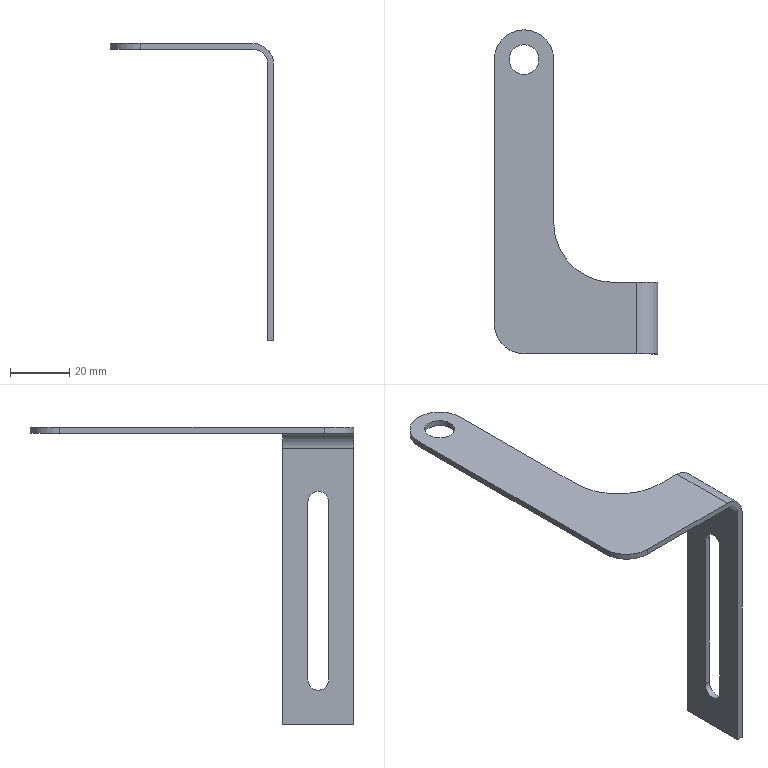Part | STEP file | 冲床-300配套压波_id558_x_t | 1 solid | 20 faces | box 55 x 109 x 100 mm | volume 9589 mm3 | plane 11 | cylinder 9 | commonest cylinder face diameters 20 x3 7 x2 10 x2 14 x1 40 x1
STEP:
#1=CARTESIAN_POINT('',(1550.,0.,165.));
#2=VERTEX_POINT('',#1);
#3=CARTESIAN_POINT('',(1550.,-55.,165.));
#4=VERTEX_POINT('',#3);
#5=CARTESIAN_POINT('',(1550.,-99.,165.));
#6=DIRECTION('',(0.,-1.,0.));
#7=VECTOR('',#6,1.);
#8=LINE('',#5,#7);
#9=EDGE_CURVE('',#2,#4,#8,.T.);
#10=ORIENTED_EDGE('',*,*,#9,.T.);
#11=CARTESIAN_POINT('',(1550.,-55.,163.));
#12=VERTEX_POINT('',#11);
#13=CARTESIAN_POINT('',(1550.,-55.,165.));
#14=DIRECTION('',(0.,0.,-1.));
#15=VECTOR('',#14,1.);
#16=LINE('',#13,#15);
#17=EDGE_CURVE('',#4,#12,#16,.T.);
#18=ORIENTED_EDGE('',*,*,#17,.T.);
#19=CARTESIAN_POINT('',(1550.,0.,163.));
#20=VERTEX_POINT('',#19);
#21=CARTESIAN_POINT('',(1550.,-99.,163.));
#22=DIRECTION('',(0.,-1.,0.));
#23=VECTOR('',#22,1.);
#24=LINE('',#21,#23);
#25=EDGE_CURVE('',#20,#12,#24,.T.);
#26=ORIENTED_EDGE('',*,*,#25,.F.);
#27=CARTESIAN_POINT('',(1550.,0.,165.));
#28=DIRECTION('',(0.,0.,1.));
#29=VECTOR('',#28,1.);
#30=LINE('',#27,#29);
#31=EDGE_CURVE('',#20,#2,#30,.T.);
#32=ORIENTED_EDGE('',*,*,#31,.T.);
#33=EDGE_LOOP('',(#10,#18,#26,#32));
#34=FACE_OUTER_BOUND('',#33,.T.);
#35=CARTESIAN_POINT('',(1550.,-99.,165.));
#36=DIRECTION('',(1.,0.,0.));
#37=DIRECTION('',(0.,1.,0.));
#38=AXIS2_PLACEMENT_3D('',#35,#36,#37);
#39=PLANE('',#38);
#40=ADVANCED_FACE('',(#34),#39,.T.);
#41=CARTESIAN_POINT('',(1530.,-89.,165.));
#42=VERTEX_POINT('',#41);
#43=CARTESIAN_POINT('',(1530.,0.,165.));
#44=VERTEX_POINT('',#43);
#45=CARTESIAN_POINT('',(1530.,-99.,165.));
#46=DIRECTION('',(0.,1.,0.));
#47=VECTOR('',#46,1.);
#48=LINE('',#45,#47);
#49=EDGE_CURVE('',#42,#44,#48,.T.);
#50=ORIENTED_EDGE('',*,*,#49,.T.);
#51=CARTESIAN_POINT('',(1530.,0.,163.));
#52=VERTEX_POINT('',#51);
#53=CARTESIAN_POINT('',(1530.,0.,165.));
#54=DIRECTION('',(0.,0.,-1.));
#55=VECTOR('',#54,1.);
#56=LINE('',#53,#55);
#57=EDGE_CURVE('',#44,#52,#56,.T.);
#58=ORIENTED_EDGE('',*,*,#57,.T.);
#59=CARTESIAN_POINT('',(1530.,-89.,163.));
#60=VERTEX_POINT('',#59);
#61=CARTESIAN_POINT('',(1530.,-99.,163.));
#62=DIRECTION('',(0.,1.,0.));
#63=VECTOR('',#62,1.);
#64=LINE('',#61,#63);
#65=EDGE_CURVE('',#60,#52,#64,.T.);
#66=ORIENTED_EDGE('',*,*,#65,.F.);
#67=CARTESIAN_POINT('',(1530.,-89.,165.));
#68=DIRECTION('',(0.,0.,1.));
#69=VECTOR('',#68,1.);
#70=LINE('',#67,#69);
#71=EDGE_CURVE('',#60,#42,#70,.T.);
#72=ORIENTED_EDGE('',*,*,#71,.T.);
#73=EDGE_LOOP('',(#50,#58,#66,#72));
#74=FACE_OUTER_BOUND('',#73,.T.);
#75=CARTESIAN_POINT('',(1530.,-99.,165.));
#76=DIRECTION('',(1.,0.,0.));
#77=DIRECTION('',(0.,1.,0.));
#78=AXIS2_PLACEMENT_3D('',#75,#76,#77);
#79=PLANE('',#78);
#80=ADVANCED_FACE('',(#74),#79,.F.);
#81=CARTESIAN_POINT('',(1578.,-99.,163.));
#82=VERTEX_POINT('',#81);
#83=CARTESIAN_POINT('',(1540.,-99.,163.));
#84=VERTEX_POINT('',#83);
#85=CARTESIAN_POINT('',(1585.,-99.,163.));
#86=DIRECTION('',(-1.,0.,0.));
#87=VECTOR('',#86,1.);
#88=LINE('',#85,#87);
#89=EDGE_CURVE('',#82,#84,#88,.T.);
#90=ORIENTED_EDGE('',*,*,#89,.F.);
#91=CARTESIAN_POINT('',(1583.,-99.,158.));
#92=VERTEX_POINT('',#91);
#93=CARTESIAN_POINT('',(1578.,-99.,158.));
#94=DIRECTION('',(0.,1.,0.));
#95=DIRECTION('',(-1.,0.,0.));
#96=AXIS2_PLACEMENT_3D('',#93,#94,#95);
#97=CIRCLE('',#96,5.);
#98=EDGE_CURVE('',#82,#92,#97,.T.);
#99=ORIENTED_EDGE('',*,*,#98,.T.);
#100=CARTESIAN_POINT('',(1583.,-99.,65.));
#101=VERTEX_POINT('',#100);
#102=CARTESIAN_POINT('',(1583.,-99.,0.));
#103=DIRECTION('',(0.,0.,1.));
#104=VECTOR('',#103,1.);
#105=LINE('',#102,#104);
#106=EDGE_CURVE('',#101,#92,#105,.T.);
#107=ORIENTED_EDGE('',*,*,#106,.F.);
#108=CARTESIAN_POINT('',(1585.,-99.,65.));
#109=VERTEX_POINT('',#108);
#110=CARTESIAN_POINT('',(1585.,-99.,65.));
#111=DIRECTION('',(-1.,0.,0.));
#112=VECTOR('',#111,1.);
#113=LINE('',#110,#112);
#114=EDGE_CURVE('',#109,#101,#113,.T.);
#115=ORIENTED_EDGE('',*,*,#114,.F.);
#116=CARTESIAN_POINT('',(1585.,-99.,158.));
#117=VERTEX_POINT('',#116);
#118=CARTESIAN_POINT('',(1585.,-99.,165.));
#119=DIRECTION('',(0.,0.,1.));
#120=VECTOR('',#119,1.);
#121=LINE('',#118,#120);
#122=EDGE_CURVE('',#109,#117,#121,.T.);
#123=ORIENTED_EDGE('',*,*,#122,.T.);
#124=CARTESIAN_POINT('',(1578.,-99.,165.));
#125=VERTEX_POINT('',#124);
#126=CARTESIAN_POINT('',(1578.,-99.,158.));
#127=DIRECTION('',(0.,-1.,0.));
#128=DIRECTION('',(1.,0.,0.));
#129=AXIS2_PLACEMENT_3D('',#126,#127,#128);
#130=CIRCLE('',#129,7.);
#131=EDGE_CURVE('',#117,#125,#130,.T.);
#132=ORIENTED_EDGE('',*,*,#131,.T.);
#133=CARTESIAN_POINT('',(1540.,-99.,165.));
#134=VERTEX_POINT('',#133);
#135=CARTESIAN_POINT('',(1585.,-99.,165.));
#136=DIRECTION('',(-1.,0.,0.));
#137=VECTOR('',#136,1.);
#138=LINE('',#135,#137);
#139=EDGE_CURVE('',#125,#134,#138,.T.);
#140=ORIENTED_EDGE('',*,*,#139,.T.);
#141=CARTESIAN_POINT('',(1540.,-99.,165.));
#142=DIRECTION('',(0.,0.,-1.));
#143=VECTOR('',#142,1.);
#144=LINE('',#141,#143);
#145=EDGE_CURVE('',#134,#84,#144,.T.);
#146=ORIENTED_EDGE('',*,*,#145,.T.);
#147=EDGE_LOOP('',(#90,#99,#107,#115,#123,#132,#140,#146));
#148=FACE_OUTER_BOUND('',#147,.T.);
#149=CARTESIAN_POINT('',(1585.,-99.,165.));
#150=DIRECTION('',(0.,1.,0.));
#151=DIRECTION('',(-1.,0.,0.));
#152=AXIS2_PLACEMENT_3D('',#149,#150,#151);
#153=PLANE('',#152);
#154=ADVANCED_FACE('',(#148),#153,.F.);
#155=CARTESIAN_POINT('',(1535.,0.,163.));
#156=VERTEX_POINT('',#155);
#157=CARTESIAN_POINT('',(1540.,0.,163.));
#158=DIRECTION('',(0.,0.,-1.));
#159=DIRECTION('',(-1.,0.,0.));
#160=AXIS2_PLACEMENT_3D('',#157,#158,#159);
#161=CIRCLE('',#160,5.);
#162=EDGE_CURVE('',#156,#156,#161,.T.);
#163=ORIENTED_EDGE('',*,*,#162,.F.);
#164=EDGE_LOOP('',(#163));
#165=FACE_BOUND('',#164,.T.);
#166=ORIENTED_EDGE('',*,*,#65,.T.);
#167=CARTESIAN_POINT('',(1540.,10.,163.));
#168=VERTEX_POINT('',#167);
#169=CARTESIAN_POINT('',(1540.,0.,163.));
#170=DIRECTION('',(0.,0.,-1.));
#171=DIRECTION('',(-1.,0.,0.));
#172=AXIS2_PLACEMENT_3D('',#169,#170,#171);
#173=CIRCLE('',#172,10.);
#174=EDGE_CURVE('',#52,#168,#173,.T.);
#175=ORIENTED_EDGE('',*,*,#174,.T.);
#176=CARTESIAN_POINT('',(1540.,0.,163.));
#177=DIRECTION('',(0.,0.,-1.));
#178=DIRECTION('',(-1.,0.,0.));
#179=AXIS2_PLACEMENT_3D('',#176,#177,#178);
#180=CIRCLE('',#179,10.);
#181=EDGE_CURVE('',#168,#20,#180,.T.);
#182=ORIENTED_EDGE('',*,*,#181,.T.);
#183=ORIENTED_EDGE('',*,*,#25,.T.);
#184=CARTESIAN_POINT('',(1570.,-75.,163.));
#185=VERTEX_POINT('',#184);
#186=CARTESIAN_POINT('',(1570.,-55.,163.));
#187=DIRECTION('',(0.,0.,1.));
#188=DIRECTION('',(-1.,0.,0.));
#189=AXIS2_PLACEMENT_3D('',#186,#187,#188);
#190=CIRCLE('',#189,20.);
#191=EDGE_CURVE('',#12,#185,#190,.T.);
#192=ORIENTED_EDGE('',*,*,#191,.T.);
#193=CARTESIAN_POINT('',(1578.,-75.,163.));
#194=VERTEX_POINT('',#193);
#195=CARTESIAN_POINT('',(1585.,-75.,163.));
#196=DIRECTION('',(-1.,0.,0.));
#197=VECTOR('',#196,1.);
#198=LINE('',#195,#197);
#199=EDGE_CURVE('',#194,#185,#198,.T.);
#200=ORIENTED_EDGE('',*,*,#199,.F.);
#201=CARTESIAN_POINT('',(1578.,-99.,163.));
#202=DIRECTION('',(0.,-1.,0.));
#203=VECTOR('',#202,1.);
#204=LINE('',#201,#203);
#205=EDGE_CURVE('',#194,#82,#204,.T.);
#206=ORIENTED_EDGE('',*,*,#205,.T.);
#207=ORIENTED_EDGE('',*,*,#89,.T.);
#208=CARTESIAN_POINT('',(1540.,-89.,163.));
#209=DIRECTION('',(0.,0.,-1.));
#210=DIRECTION('',(-1.,0.,0.));
#211=AXIS2_PLACEMENT_3D('',#208,#209,#210);
#212=CIRCLE('',#211,10.);
#213=EDGE_CURVE('',#84,#60,#212,.T.);
#214=ORIENTED_EDGE('',*,*,#213,.T.);
#215=EDGE_LOOP('',(#166,#175,#182,#183,#192,#200,#206,#207,#214));
#216=FACE_BOUND('',#215,.T.);
#217=CARTESIAN_POINT('',(1585.,-99.,163.));
#218=DIRECTION('',(0.,0.,-1.));
#219=DIRECTION('',(-1.,0.,0.));
#220=AXIS2_PLACEMENT_3D('',#217,#218,#219);
#221=PLANE('',#220);
#222=ADVANCED_FACE('',(#165,#216),#221,.T.);
#223=CARTESIAN_POINT('',(1535.,0.,165.));
#224=VERTEX_POINT('',#223);
#225=CARTESIAN_POINT('',(1540.,0.,165.));
#226=DIRECTION('',(0.,0.,-1.));
#227=DIRECTION('',(-1.,0.,0.));
#228=AXIS2_PLACEMENT_3D('',#225,#226,#227);
#229=CIRCLE('',#228,5.);
#230=EDGE_CURVE('',#224,#224,#229,.T.);
#231=ORIENTED_EDGE('',*,*,#230,.T.);
#232=EDGE_LOOP('',(#231));
#233=FACE_BOUND('',#232,.T.);
#234=ORIENTED_EDGE('',*,*,#139,.F.);
#235=CARTESIAN_POINT('',(1578.,-75.,165.));
#236=VERTEX_POINT('',#235);
#237=CARTESIAN_POINT('',(1578.,-99.,165.));
#238=DIRECTION('',(0.,1.,0.));
#239=VECTOR('',#238,1.);
#240=LINE('',#237,#239);
#241=EDGE_CURVE('',#125,#236,#240,.T.);
#242=ORIENTED_EDGE('',*,*,#241,.T.);
#243=CARTESIAN_POINT('',(1570.,-75.,165.));
#244=VERTEX_POINT('',#243);
#245=CARTESIAN_POINT('',(1583.,-75.,165.));
#246=DIRECTION('',(-1.,0.,0.));
#247=VECTOR('',#246,1.);
#248=LINE('',#245,#247);
#249=EDGE_CURVE('',#236,#244,#248,.T.);
#250=ORIENTED_EDGE('',*,*,#249,.T.);
#251=CARTESIAN_POINT('',(1570.,-55.,165.));
#252=DIRECTION('',(0.,0.,-1.));
#253=DIRECTION('',(-1.,0.,0.));
#254=AXIS2_PLACEMENT_3D('',#251,#252,#253);
#255=CIRCLE('',#254,20.);
#256=EDGE_CURVE('',#244,#4,#255,.T.);
#257=ORIENTED_EDGE('',*,*,#256,.T.);
#258=ORIENTED_EDGE('',*,*,#9,.F.);
#259=CARTESIAN_POINT('',(1540.,10.,165.));
#260=VERTEX_POINT('',#259);
#261=CARTESIAN_POINT('',(1540.,0.,165.));
#262=DIRECTION('',(0.,0.,1.));
#263=DIRECTION('',(-1.,0.,0.));
#264=AXIS2_PLACEMENT_3D('',#261,#262,#263);
#265=CIRCLE('',#264,10.);
#266=EDGE_CURVE('',#2,#260,#265,.T.);
#267=ORIENTED_EDGE('',*,*,#266,.T.);
#268=CARTESIAN_POINT('',(1540.,0.,165.));
#269=DIRECTION('',(0.,0.,1.));
#270=DIRECTION('',(-1.,0.,0.));
#271=AXIS2_PLACEMENT_3D('',#268,#269,#270);
#272=CIRCLE('',#271,10.);
#273=EDGE_CURVE('',#260,#44,#272,.T.);
#274=ORIENTED_EDGE('',*,*,#273,.T.);
#275=ORIENTED_EDGE('',*,*,#49,.F.);
#276=CARTESIAN_POINT('',(1540.,-89.,165.));
#277=DIRECTION('',(0.,0.,1.));
#278=DIRECTION('',(-1.,0.,0.));
#279=AXIS2_PLACEMENT_3D('',#276,#277,#278);
#280=CIRCLE('',#279,10.);
#281=EDGE_CURVE('',#42,#134,#280,.T.);
#282=ORIENTED_EDGE('',*,*,#281,.T.);
#283=EDGE_LOOP('',(#234,#242,#250,#257,#258,#267,#274,#275,#282));
#284=FACE_BOUND('',#283,.T.);
#285=CARTESIAN_POINT('',(1585.,-99.,165.));
#286=DIRECTION('',(0.,0.,-1.));
#287=DIRECTION('',(-1.,0.,0.));
#288=AXIS2_PLACEMENT_3D('',#285,#286,#287);
#289=PLANE('',#288);
#290=ADVANCED_FACE('',(#233,#284),#289,.F.);
#291=CARTESIAN_POINT('',(1585.,-75.,158.));
#292=VERTEX_POINT('',#291);
#293=CARTESIAN_POINT('',(1585.,-75.,65.));
#294=VERTEX_POINT('',#293);
#295=CARTESIAN_POINT('',(1585.,-75.,20.));
#296=DIRECTION('',(0.,0.,-1.));
#297=VECTOR('',#296,1.);
#298=LINE('',#295,#297);
#299=EDGE_CURVE('',#292,#294,#298,.T.);
#300=ORIENTED_EDGE('',*,*,#299,.T.);
#301=CARTESIAN_POINT('',(1583.,-75.,65.));
#302=VERTEX_POINT('',#301);
#303=CARTESIAN_POINT('',(1583.,-75.,65.));
#304=DIRECTION('',(-1.,0.,0.));
#305=VECTOR('',#304,1.);
#306=LINE('',#303,#305);
#307=EDGE_CURVE('',#294,#302,#306,.T.);
#308=ORIENTED_EDGE('',*,*,#307,.T.);
#309=CARTESIAN_POINT('',(1583.,-75.,158.));
#310=VERTEX_POINT('',#309);
#311=CARTESIAN_POINT('',(1583.,-75.,20.));
#312=DIRECTION('',(0.,0.,-1.));
#313=VECTOR('',#312,1.);
#314=LINE('',#311,#313);
#315=EDGE_CURVE('',#310,#302,#314,.T.);
#316=ORIENTED_EDGE('',*,*,#315,.F.);
#317=CARTESIAN_POINT('',(1578.,-75.,158.));
#318=DIRECTION('',(0.,-1.,0.));
#319=DIRECTION('',(1.,0.,0.));
#320=AXIS2_PLACEMENT_3D('',#317,#318,#319);
#321=CIRCLE('',#320,5.);
#322=EDGE_CURVE('',#310,#194,#321,.T.);
#323=ORIENTED_EDGE('',*,*,#322,.T.);
#324=ORIENTED_EDGE('',*,*,#199,.T.);
#325=CARTESIAN_POINT('',(1570.,-75.,20.));
#326=DIRECTION('',(0.,0.,1.));
#327=VECTOR('',#326,1.);
#328=LINE('',#325,#327);
#329=EDGE_CURVE('',#185,#244,#328,.T.);
#330=ORIENTED_EDGE('',*,*,#329,.T.);
#331=ORIENTED_EDGE('',*,*,#249,.F.);
#332=CARTESIAN_POINT('',(1578.,-75.,158.));
#333=DIRECTION('',(0.,1.,0.));
#334=DIRECTION('',(-1.,0.,0.));
#335=AXIS2_PLACEMENT_3D('',#332,#333,#334);
#336=CIRCLE('',#335,7.);
#337=EDGE_CURVE('',#236,#292,#336,.T.);
#338=ORIENTED_EDGE('',*,*,#337,.T.);
#339=EDGE_LOOP('',(#300,#308,#316,#323,#324,#330,#331,#338));
#340=FACE_OUTER_BOUND('',#339,.T.);
#341=CARTESIAN_POINT('',(1583.,-75.,20.));
#342=DIRECTION('',(0.,-1.,0.));
#343=DIRECTION('',(-1.,0.,0.));
#344=AXIS2_PLACEMENT_3D('',#341,#342,#343);
#345=PLANE('',#344);
#346=ADVANCED_FACE('',(#340),#345,.F.);
#347=CARTESIAN_POINT('',(1585.,-99.,65.));
#348=DIRECTION('',(0.,-1.,0.));
#349=VECTOR('',#348,1.);
#350=LINE('',#347,#349);
#351=EDGE_CURVE('',#294,#109,#350,.T.);
#352=ORIENTED_EDGE('',*,*,#351,.T.);
#353=ORIENTED_EDGE('',*,*,#114,.T.);
#354=CARTESIAN_POINT('',(1583.,-99.,65.));
#355=DIRECTION('',(0.,-1.,0.));
#356=VECTOR('',#355,1.);
#357=LINE('',#354,#356);
#358=EDGE_CURVE('',#302,#101,#357,.T.);
#359=ORIENTED_EDGE('',*,*,#358,.F.);
#360=ORIENTED_EDGE('',*,*,#307,.F.);
#361=EDGE_LOOP('',(#352,#353,#359,#360));
#362=FACE_OUTER_BOUND('',#361,.T.);
#363=CARTESIAN_POINT('',(1583.,-99.,65.));
#364=DIRECTION('',(0.,0.,1.));
#365=DIRECTION('',(1.,0.,0.));
#366=AXIS2_PLACEMENT_3D('',#363,#364,#365);
#367=PLANE('',#366);
#368=ADVANCED_FACE('',(#362),#367,.F.);
#369=CARTESIAN_POINT('',(1583.,-83.5,140.));
#370=VERTEX_POINT('',#369);
#371=CARTESIAN_POINT('',(1583.,-90.5,140.));
#372=VERTEX_POINT('',#371);
#373=CARTESIAN_POINT('',(1583.,-87.,140.));
#374=DIRECTION('',(1.,0.,0.));
#375=DIRECTION('',(0.,-1.,0.));
#376=AXIS2_PLACEMENT_3D('',#373,#374,#375);
#377=CIRCLE('',#376,3.5);
#378=EDGE_CURVE('',#370,#372,#377,.T.);
#379=ORIENTED_EDGE('',*,*,#378,.T.);
#380=CARTESIAN_POINT('',(1583.,-90.5,80.));
#381=VERTEX_POINT('',#380);
#382=CARTESIAN_POINT('',(1583.,-90.5,0.));
#383=DIRECTION('',(0.,0.,-1.));
#384=VECTOR('',#383,1.);
#385=LINE('',#382,#384);
#386=EDGE_CURVE('',#372,#381,#385,.T.);
#387=ORIENTED_EDGE('',*,*,#386,.T.);
#388=CARTESIAN_POINT('',(1583.,-83.5,80.));
#389=VERTEX_POINT('',#388);
#390=CARTESIAN_POINT('',(1583.,-87.,80.));
#391=DIRECTION('',(1.,0.,0.));
#392=DIRECTION('',(0.,-1.,0.));
#393=AXIS2_PLACEMENT_3D('',#390,#391,#392);
#394=CIRCLE('',#393,3.5);
#395=EDGE_CURVE('',#381,#389,#394,.T.);
#396=ORIENTED_EDGE('',*,*,#395,.T.);
#397=CARTESIAN_POINT('',(1583.,-83.5,0.));
#398=DIRECTION('',(0.,0.,1.));
#399=VECTOR('',#398,1.);
#400=LINE('',#397,#399);
#401=EDGE_CURVE('',#389,#370,#400,.T.);
#402=ORIENTED_EDGE('',*,*,#401,.T.);
#403=EDGE_LOOP('',(#379,#387,#396,#402));
#404=FACE_BOUND('',#403,.T.);
#405=ORIENTED_EDGE('',*,*,#315,.T.);
#406=ORIENTED_EDGE('',*,*,#358,.T.);
#407=ORIENTED_EDGE('',*,*,#106,.T.);
#408=CARTESIAN_POINT('',(1583.,0.,158.));
#409=DIRECTION('',(0.,1.,0.));
#410=VECTOR('',#409,1.);
#411=LINE('',#408,#410);
#412=EDGE_CURVE('',#92,#310,#411,.T.);
#413=ORIENTED_EDGE('',*,*,#412,.T.);
#414=EDGE_LOOP('',(#405,#406,#407,#413));
#415=FACE_BOUND('',#414,.T.);
#416=CARTESIAN_POINT('',(1583.,0.,0.));
#417=DIRECTION('',(-1.,0.,0.));
#418=DIRECTION('',(0.,0.,1.));
#419=AXIS2_PLACEMENT_3D('',#416,#417,#418);
#420=PLANE('',#419);
#421=ADVANCED_FACE('',(#404,#415),#420,.T.);
#422=CARTESIAN_POINT('',(1585.,-83.5,80.));
#423=VERTEX_POINT('',#422);
#424=CARTESIAN_POINT('',(1585.,-83.5,140.));
#425=VERTEX_POINT('',#424);
#426=CARTESIAN_POINT('',(1585.,-83.5,0.));
#427=DIRECTION('',(0.,0.,1.));
#428=VECTOR('',#427,1.);
#429=LINE('',#426,#428);
#430=EDGE_CURVE('',#423,#425,#429,.T.);
#431=ORIENTED_EDGE('',*,*,#430,.F.);
#432=CARTESIAN_POINT('',(1585.,-90.5,80.));
#433=VERTEX_POINT('',#432);
#434=CARTESIAN_POINT('',(1585.,-87.,80.));
#435=DIRECTION('',(1.,0.,0.));
#436=DIRECTION('',(0.,0.,1.));
#437=AXIS2_PLACEMENT_3D('',#434,#435,#436);
#438=CIRCLE('',#437,3.5);
#439=EDGE_CURVE('',#433,#423,#438,.T.);
#440=ORIENTED_EDGE('',*,*,#439,.F.);
#441=CARTESIAN_POINT('',(1585.,-90.5,140.));
#442=VERTEX_POINT('',#441);
#443=CARTESIAN_POINT('',(1585.,-90.5,0.));
#444=DIRECTION('',(0.,0.,-1.));
#445=VECTOR('',#444,1.);
#446=LINE('',#443,#445);
#447=EDGE_CURVE('',#442,#433,#446,.T.);
#448=ORIENTED_EDGE('',*,*,#447,.F.);
#449=CARTESIAN_POINT('',(1585.,-87.,140.));
#450=DIRECTION('',(1.,0.,0.));
#451=DIRECTION('',(0.,0.,1.));
#452=AXIS2_PLACEMENT_3D('',#449,#450,#451);
#453=CIRCLE('',#452,3.5);
#454=EDGE_CURVE('',#425,#442,#453,.T.);
#455=ORIENTED_EDGE('',*,*,#454,.F.);
#456=EDGE_LOOP('',(#431,#440,#448,#455));
#457=FACE_BOUND('',#456,.T.);
#458=ORIENTED_EDGE('',*,*,#122,.F.);
#459=ORIENTED_EDGE('',*,*,#351,.F.);
#460=ORIENTED_EDGE('',*,*,#299,.F.);
#461=CARTESIAN_POINT('',(1585.,0.,158.));
#462=DIRECTION('',(0.,-1.,0.));
#463=VECTOR('',#462,1.);
#464=LINE('',#461,#463);
#465=EDGE_CURVE('',#292,#117,#464,.T.);
#466=ORIENTED_EDGE('',*,*,#465,.T.);
#467=EDGE_LOOP('',(#458,#459,#460,#466));
#468=FACE_BOUND('',#467,.T.);
#469=CARTESIAN_POINT('',(1585.,0.,0.));
#470=DIRECTION('',(-1.,0.,0.));
#471=DIRECTION('',(0.,0.,1.));
#472=AXIS2_PLACEMENT_3D('',#469,#470,#471);
#473=PLANE('',#472);
#474=ADVANCED_FACE('',(#457,#468),#473,.F.);
#475=ORIENTED_EDGE('',*,*,#191,.F.);
#476=ORIENTED_EDGE('',*,*,#17,.F.);
#477=ORIENTED_EDGE('',*,*,#256,.F.);
#478=ORIENTED_EDGE('',*,*,#329,.F.);
#479=EDGE_LOOP('',(#475,#476,#477,#478));
#480=FACE_OUTER_BOUND('',#479,.T.);
#481=CARTESIAN_POINT('',(1570.,-55.,165.));
#482=DIRECTION('',(0.,0.,1.));
#483=DIRECTION('',(1.,0.,0.));
#484=AXIS2_PLACEMENT_3D('',#481,#482,#483);
#485=CYLINDRICAL_SURFACE('',#484,20.);
#486=ADVANCED_FACE('',(#480),#485,.F.);
#487=ORIENTED_EDGE('',*,*,#31,.F.);
#488=ORIENTED_EDGE('',*,*,#181,.F.);
#489=CARTESIAN_POINT('',(1540.,10.,165.));
#490=DIRECTION('',(0.,0.,-1.));
#491=VECTOR('',#490,1.);
#492=LINE('',#489,#491);
#493=EDGE_CURVE('',#260,#168,#492,.T.);
#494=ORIENTED_EDGE('',*,*,#493,.F.);
#495=ORIENTED_EDGE('',*,*,#266,.F.);
#496=EDGE_LOOP('',(#487,#488,#494,#495));
#497=FACE_OUTER_BOUND('',#496,.T.);
#498=CARTESIAN_POINT('',(1540.,0.,165.));
#499=DIRECTION('',(0.,0.,-1.));
#500=DIRECTION('',(-1.,0.,0.));
#501=AXIS2_PLACEMENT_3D('',#498,#499,#500);
#502=CYLINDRICAL_SURFACE('',#501,10.);
#503=ADVANCED_FACE('',(#497),#502,.T.);
#504=ORIENTED_EDGE('',*,*,#273,.F.);
#505=ORIENTED_EDGE('',*,*,#493,.T.);
#506=ORIENTED_EDGE('',*,*,#174,.F.);
#507=ORIENTED_EDGE('',*,*,#57,.F.);
#508=EDGE_LOOP('',(#504,#505,#506,#507));
#509=FACE_OUTER_BOUND('',#508,.T.);
#510=CARTESIAN_POINT('',(1540.,0.,165.));
#511=DIRECTION('',(0.,0.,1.));
#512=DIRECTION('',(1.,0.,0.));
#513=AXIS2_PLACEMENT_3D('',#510,#511,#512);
#514=CYLINDRICAL_SURFACE('',#513,10.);
#515=ADVANCED_FACE('',(#509),#514,.T.);
#516=ORIENTED_EDGE('',*,*,#98,.F.);
#517=ORIENTED_EDGE('',*,*,#205,.F.);
#518=ORIENTED_EDGE('',*,*,#322,.F.);
#519=ORIENTED_EDGE('',*,*,#412,.F.);
#520=EDGE_LOOP('',(#516,#517,#518,#519));
#521=FACE_OUTER_BOUND('',#520,.T.);
#522=CARTESIAN_POINT('',(1578.,-99.,158.));
#523=DIRECTION('',(0.,-1.,0.));
#524=DIRECTION('',(0.,0.,1.));
#525=AXIS2_PLACEMENT_3D('',#522,#523,#524);
#526=CYLINDRICAL_SURFACE('',#525,5.);
#527=ADVANCED_FACE('',(#521),#526,.F.);
#528=ORIENTED_EDGE('',*,*,#337,.F.);
#529=ORIENTED_EDGE('',*,*,#241,.F.);
#530=ORIENTED_EDGE('',*,*,#131,.F.);
#531=ORIENTED_EDGE('',*,*,#465,.F.);
#532=EDGE_LOOP('',(#528,#529,#530,#531));
#533=FACE_OUTER_BOUND('',#532,.T.);
#534=CARTESIAN_POINT('',(1578.,-99.,158.));
#535=DIRECTION('',(0.,-1.,0.));
#536=DIRECTION('',(0.,0.,1.));
#537=AXIS2_PLACEMENT_3D('',#534,#535,#536);
#538=CYLINDRICAL_SURFACE('',#537,7.);
#539=ADVANCED_FACE('',(#533),#538,.T.);
#540=CARTESIAN_POINT('',(1556.,-83.5,140.));
#541=DIRECTION('',(1.,0.,0.));
#542=VECTOR('',#541,1.);
#543=LINE('',#540,#542);
#544=EDGE_CURVE('',#370,#425,#543,.T.);
#545=ORIENTED_EDGE('',*,*,#544,.F.);
#546=ORIENTED_EDGE('',*,*,#401,.F.);
#547=CARTESIAN_POINT('',(1556.,-83.5,80.));
#548=DIRECTION('',(1.,0.,0.));
#549=VECTOR('',#548,1.);
#550=LINE('',#547,#549);
#551=EDGE_CURVE('',#389,#423,#550,.T.);
#552=ORIENTED_EDGE('',*,*,#551,.T.);
#553=ORIENTED_EDGE('',*,*,#430,.T.);
#554=EDGE_LOOP('',(#545,#546,#552,#553));
#555=FACE_OUTER_BOUND('',#554,.T.);
#556=CARTESIAN_POINT('',(1556.,-83.5,80.));
#557=DIRECTION('',(0.,-1.,0.));
#558=DIRECTION('',(0.,0.,1.));
#559=AXIS2_PLACEMENT_3D('',#556,#557,#558);
#560=PLANE('',#559);
#561=ADVANCED_FACE('',(#555),#560,.T.);
#562=CARTESIAN_POINT('',(1556.,-90.5,140.));
#563=DIRECTION('',(1.,0.,0.));
#564=VECTOR('',#563,1.);
#565=LINE('',#562,#564);
#566=EDGE_CURVE('',#372,#442,#565,.T.);
#567=ORIENTED_EDGE('',*,*,#566,.F.);
#568=ORIENTED_EDGE('',*,*,#378,.F.);
#569=ORIENTED_EDGE('',*,*,#544,.T.);
#570=ORIENTED_EDGE('',*,*,#454,.T.);
#571=EDGE_LOOP('',(#567,#568,#569,#570));
#572=FACE_OUTER_BOUND('',#571,.T.);
#573=CARTESIAN_POINT('',(1556.,-87.,140.));
#574=DIRECTION('',(1.,0.,0.));
#575=DIRECTION('',(0.,0.,-1.));
#576=AXIS2_PLACEMENT_3D('',#573,#574,#575);
#577=CYLINDRICAL_SURFACE('',#576,3.5);
#578=ADVANCED_FACE('',(#572),#577,.F.);
#579=CARTESIAN_POINT('',(1556.,-90.5,80.));
#580=DIRECTION('',(1.,0.,0.));
#581=VECTOR('',#580,1.);
#582=LINE('',#579,#581);
#583=EDGE_CURVE('',#381,#433,#582,.T.);
#584=ORIENTED_EDGE('',*,*,#583,.F.);
#585=ORIENTED_EDGE('',*,*,#386,.F.);
#586=ORIENTED_EDGE('',*,*,#566,.T.);
#587=ORIENTED_EDGE('',*,*,#447,.T.);
#588=EDGE_LOOP('',(#584,#585,#586,#587));
#589=FACE_OUTER_BOUND('',#588,.T.);
#590=CARTESIAN_POINT('',(1556.,-90.5,140.));
#591=DIRECTION('',(0.,1.,0.));
#592=DIRECTION('',(0.,0.,-1.));
#593=AXIS2_PLACEMENT_3D('',#590,#591,#592);
#594=PLANE('',#593);
#595=ADVANCED_FACE('',(#589),#594,.T.);
#596=ORIENTED_EDGE('',*,*,#551,.F.);
#597=ORIENTED_EDGE('',*,*,#395,.F.);
#598=ORIENTED_EDGE('',*,*,#583,.T.);
#599=ORIENTED_EDGE('',*,*,#439,.T.);
#600=EDGE_LOOP('',(#596,#597,#598,#599));
#601=FACE_OUTER_BOUND('',#600,.T.);
#602=CARTESIAN_POINT('',(1556.,-87.,80.));
#603=DIRECTION('',(1.,0.,0.));
#604=DIRECTION('',(0.,0.,-1.));
#605=AXIS2_PLACEMENT_3D('',#602,#603,#604);
#606=CYLINDRICAL_SURFACE('',#605,3.5);
#607=ADVANCED_FACE('',(#601),#606,.F.);
#608=ORIENTED_EDGE('',*,*,#281,.F.);
#609=ORIENTED_EDGE('',*,*,#71,.F.);
#610=ORIENTED_EDGE('',*,*,#213,.F.);
#611=ORIENTED_EDGE('',*,*,#145,.F.);
#612=EDGE_LOOP('',(#608,#609,#610,#611));
#613=FACE_OUTER_BOUND('',#612,.T.);
#614=CARTESIAN_POINT('',(1540.,-89.,165.));
#615=DIRECTION('',(0.,0.,-1.));
#616=DIRECTION('',(-1.,0.,0.));
#617=AXIS2_PLACEMENT_3D('',#614,#615,#616);
#618=CYLINDRICAL_SURFACE('',#617,10.);
#619=ADVANCED_FACE('',(#613),#618,.T.);
#620=ORIENTED_EDGE('',*,*,#162,.T.);
#621=EDGE_LOOP('',(#620));
#622=FACE_BOUND('',#621,.T.);
#623=ORIENTED_EDGE('',*,*,#230,.F.);
#624=EDGE_LOOP('',(#623));
#625=FACE_BOUND('',#624,.T.);
#626=CARTESIAN_POINT('',(1540.,0.,180.06));
#627=DIRECTION('',(0.,0.,-1.));
#628=DIRECTION('',(0.,-1.,0.));
#629=AXIS2_PLACEMENT_3D('',#626,#627,#628);
#630=CYLINDRICAL_SURFACE('',#629,5.);
#631=ADVANCED_FACE('',(#622,#625),#630,.F.);
#632=CLOSED_SHELL('',(#40,#80,#154,#222,#290,#346,#368,#421,#474,#486,#503,#515,#527,#539,#561,#578,#595,#607,#619,#631));
#633=MANIFOLD_SOLID_BREP('',#632);
#634=(LENGTH_UNIT()NAMED_UNIT(*)SI_UNIT(.MILLI.,.METRE.));
#635=UNCERTAINTY_MEASURE_WITH_UNIT(LENGTH_MEASURE(0.00002),#634,'','');
#636=(NAMED_UNIT(*)PLANE_ANGLE_UNIT()SI_UNIT($,.RADIAN.));
#637=PLANE_ANGLE_MEASURE_WITH_UNIT(PLANE_ANGLE_MEASURE(0.01745),#636);
#638=DIMENSIONAL_EXPONENTS(0.,0.,0.,0.,0.,0.,0.);
#639=(CONVERSION_BASED_UNIT('DEGREE',#637)NAMED_UNIT(#638)PLANE_ANGLE_UNIT());
#640=(NAMED_UNIT(*)SI_UNIT($,.STERADIAN.)SOLID_ANGLE_UNIT());
#641=(GEOMETRIC_REPRESENTATION_CONTEXT(3)GLOBAL_UNCERTAINTY_ASSIGNED_CONTEXT((#635))GLOBAL_UNIT_ASSIGNED_CONTEXT((#634,#639,#640))REPRESENTATION_CONTEXT('',''));
#642=ADVANCED_BREP_SHAPE_REPRESENTATION('',(#633),#641);